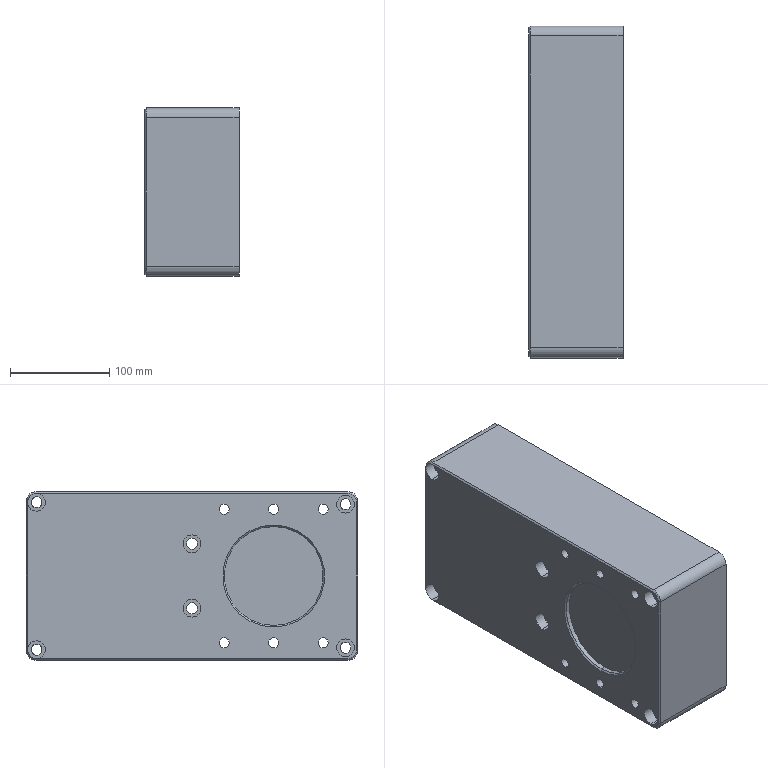Part | SolidWorks | features HoleWzd 3, MirrorPattern 3, Chamfer 2, Fillet 2, ICE 2, Extrusion 1 | 1 solid | 72 faces | box 95 x 335 x 170 mm | volume 1808811 mm3 | cylinder 42 | plane 24 | cone 6 | commonest cylinder face diameters 10.2 x12 11 x12 18 x12 20 x4 100 x2